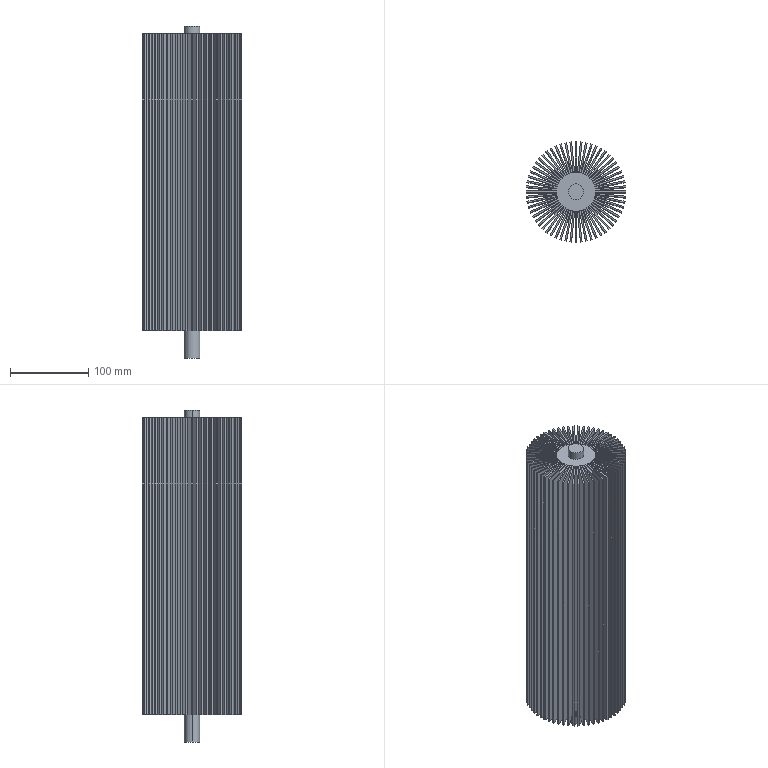Part | SolidWorks | features ICE 3, CirPattern 1, Extrusion 1 | 1 solid | 248 faces | box 128 x 128 x 425 mm | volume 2538969 mm3 | plane 184 | cylinder 64 | commonest cylinder face diameters 50 x60 20 x4